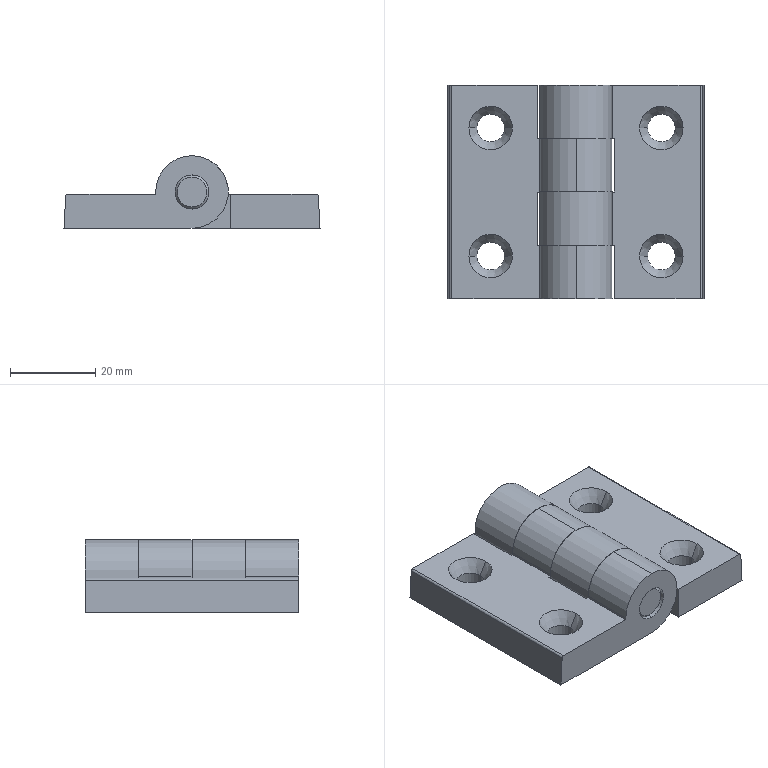Part | STEP file | LE-NHY-40_LE0314013112 | 3 solids | 64 faces | box 60 x 50 x 17 mm | volume 27546 mm3 | cylinder 26 | plane 26 | cone 12 | commonest cylinder face diameters 8 x10 6.5 x8 17 x6 1 x2